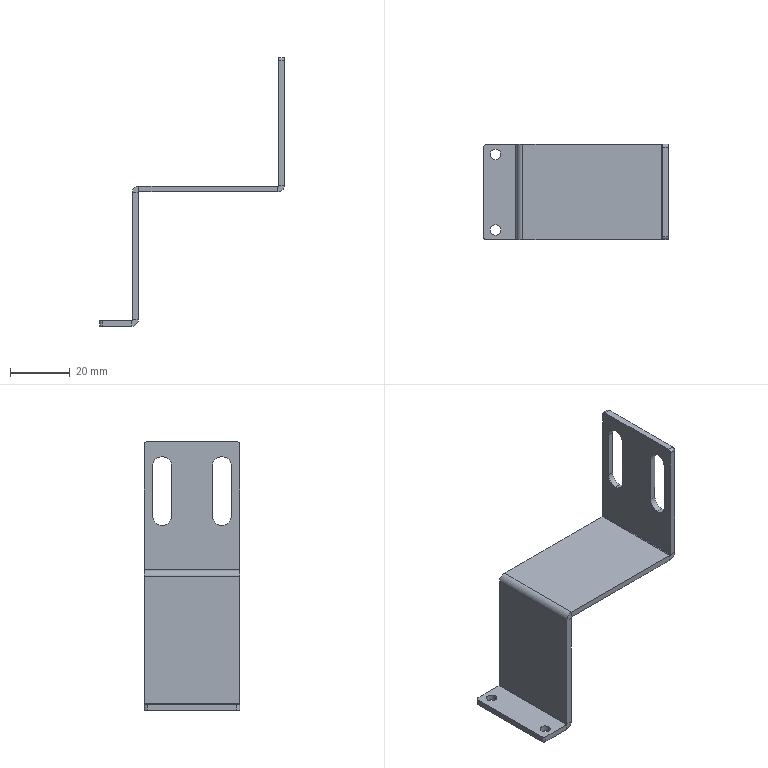Part | STEP file | 1 solid | 48 faces | box 62 x 32 x 90 mm | volume 8899 mm3 | plane 28 | cylinder 20 | commonest cylinder face diameters 6.5 x6 2 x4 3.5 x4 0.4 x3 4.4 x3